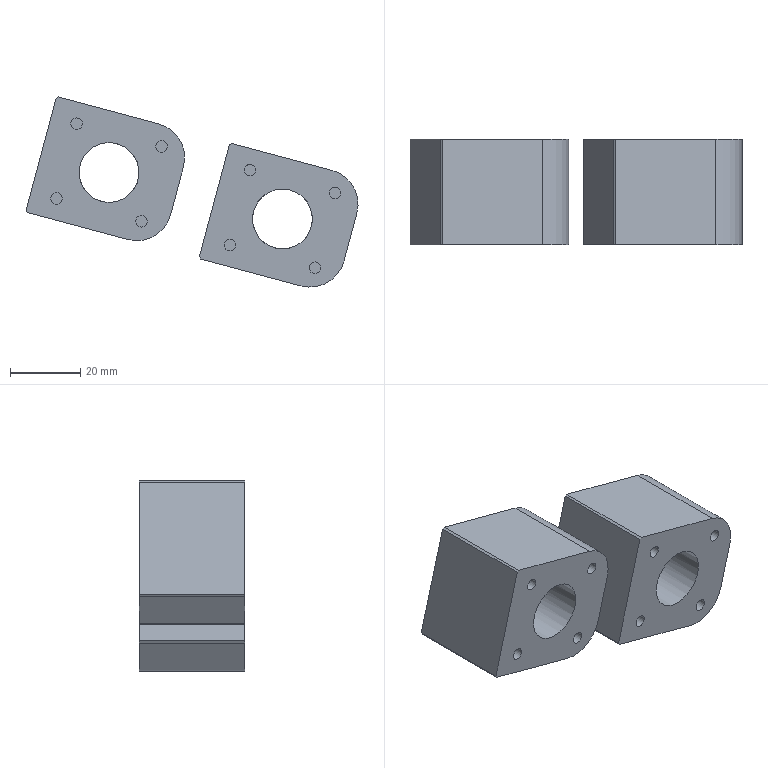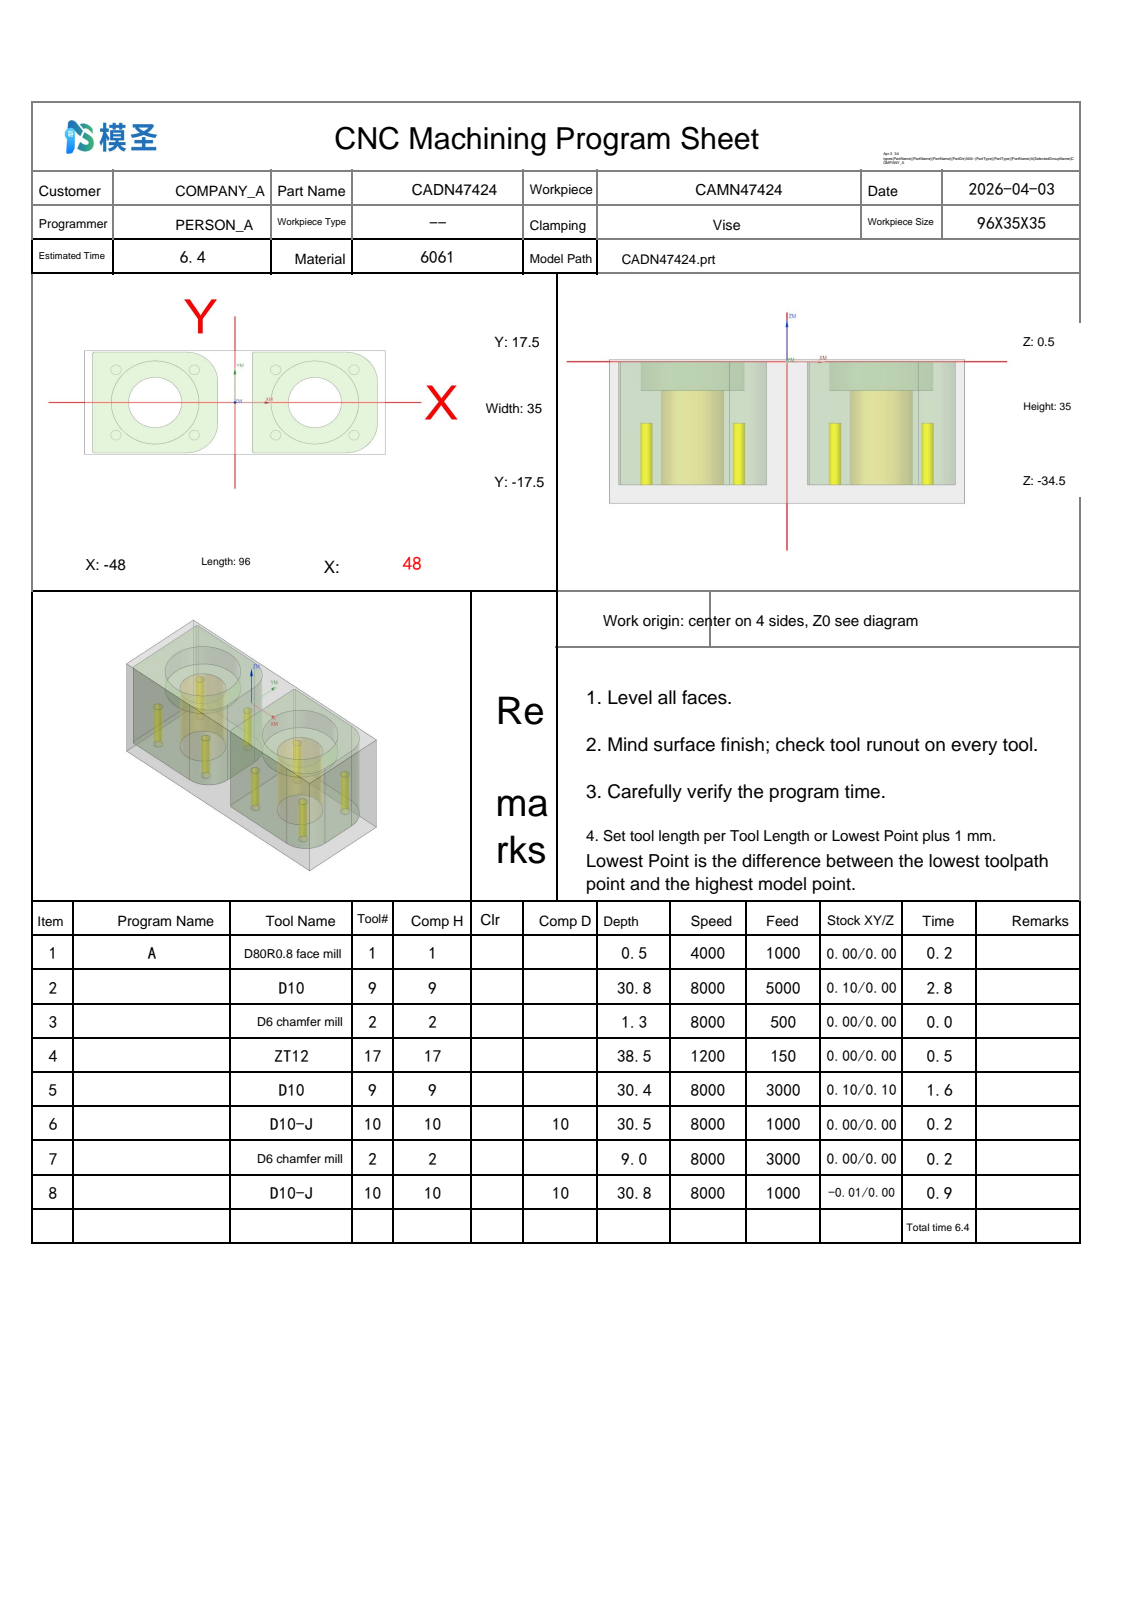NC program | NX | posted by the shop | part box 94.322 x 30 x 54.017 mm
Lines 1 to 1042 of 2047:
%
O0001
(Machine time: 8.07 MIN)
(===Total Tool:5===)
(T1=D80R0.8 face mill D=80.  R=0.8  D-  H01 Z=-0.   )
(T9=D10     D=10.  R=0.   D-  H09 Z=-30.3 )
(T2=D6 chamfer mill   D=6.   R=0.   D-  H02 Z=-8.5  )
(T17=ZT12   D=12.  DR_a=118 D-  H17 Z=-38.  )
(T10=D10-J  D=10.  R=0.   D10 H10 Z=-30.3 )
G80 G90 G17 G49 G40
G91 G28 Z0
M01
N1 T01 M06
(D80R0.8 face mill  D=80. R=0.8 H=01 ce=0.00 di=0.00)
G00 G90 G54 X90.5 Y0.0 M03 S4000
G43 H01 Z20.
M08
Z2.
G01 Z0.0 F1000.
X85.5
X-85.5
X-90.5
Z2.
G00 Z20.
G91 G28 Z0.0
M05
M09
G91 G28 Z0.0
M01
N2 T09 M06
(D10  D=10. R=0. H=09 ce=0.10 di=0.00)
G00 G90 G54 X20.75 Y22.1 M03 S8000
G43 H09 Z20.
M08
Z.5
G01 X35.5 Z.432 F5000.
G02 X50.6 Y7. Z.322 I0.0 J-15.1
G01 Y-7. Z.258
G02 X35.5 Y-22.1 Z.148 I-15.1 J0.0
G01 X6. Z.012
G02 X2.394 Y-20.606 Z-.007 I0.0 J5.1
G01 X1.894 Y-20.106 Z-.01
G02 X.4 Y-16.5 Z-.029 I3.606 J3.606
G01 Y16.5 Z-.181
G02 X1.894 Y20.106 Z-.2 I5.1 J0.0
G01 X2.394 Y20.606 Z-.203
G02 X6. Y22.1 Z-.222 I3.606 J-3.606
G01 X35.5 Z-.358
G02 X50.6 Y7. Z-.468 I0.0 J-15.1
G01 Y-7. Z-.532
G02 X35.5 Y-22.1 Z-.642 I-15.1 J0.0
G01 X6. Z-.778
G02 X2.394 Y-20.606 Z-.797 I0.0 J5.1
G01 X1.894 Y-20.106 Z-.8
G02 X.4 Y-16.5 Z-.819 I3.606 J3.606
G01 Y16.5 Z-.971
G02 X1.894 Y20.106 Z-.99 I5.1 J0.0
G01 X2.394 Y20.606 Z-.993
G02 X6. Y22.1 Z-1.011 I3.606 J-3.606
G01 X35.5 Z-1.148
G02 X50.6 Y7. Z-1.257 I0.0 J-15.1
G01 Y-7. Z-1.322
G02 X35.5 Y-22.1 Z-1.432 I-15.1 J0.0
G01 X6. Z-1.568
G02 X2.394 Y-20.606 Z-1.586 I0.0 J5.1
G01 X1.894 Y-20.106 Z-1.59
G02 X.4 Y-16.5 Z-1.608 I3.606 J3.606
G01 Y16.5 Z-1.761
G02 X1.894 Y20.106 Z-1.779 I5.1 J0.0
G01 X2.394 Y20.606 Z-1.783
G02 X6. Y22.1 Z-1.801 I3.606 J-3.606
G01 X35.5 Z-1.937
G02 X50.6 Y7. Z-2.047 I0.0 J-15.1
G01 Y-7. Z-2.112
G02 X35.5 Y-22.1 Z-2.221 I-15.1 J0.0
G01 X6. Z-2.358
G02 X2.394 Y-20.606 Z-2.376 I0.0 J5.1
G01 X1.894 Y-20.106 Z-2.379
G02 X.4 Y-16.5 Z-2.398 I3.606 J3.606
G01 Y16.5 Z-2.551
G02 X1.894 Y20.106 Z-2.569 I5.1 J0.0
G01 X2.394 Y20.606 Z-2.572
G02 X6. Y22.1 Z-2.591 I3.606 J-3.606
G01 X35.5 Z-2.727
G02 X50.6 Y7. Z-2.837 I0.0 J-15.1
G01 Y-7. Z-2.901
G02 X35.5 Y-22.1 Z-3.011 I-15.1 J0.0
G01 X6. Z-3.147
G02 X2.394 Y-20.606 Z-3.166 I0.0 J5.1
G01 X1.894 Y-20.106 Z-3.169
G02 X.4 Y-16.5 Z-3.188 I3.606 J3.606
G01 Y16.5 Z-3.34
G02 X1.894 Y20.106 Z-3.359 I5.1 J0.0
G01 X2.394 Y20.606 Z-3.362
G02 X6. Y22.1 Z-3.381 I3.606 J-3.606
G01 X35.5 Z-3.517
G02 X50.6 Y7. Z-3.627 I0.0 J-15.1
G01 Y-7. Z-3.691
G02 X35.5 Y-22.1 Z-3.801 I-15.1 J0.0
G01 X6. Z-3.937
G02 X2.394 Y-20.606 Z-3.956 I0.0 J5.1
G01 X1.894 Y-20.106 Z-3.959
G02 X.4 Y-16.5 Z-3.977 I3.606 J3.606
G01 Y16.5 Z-4.13
G02 X1.894 Y20.106 Z-4.149 I5.1 J0.0
G01 X2.394 Y20.606 Z-4.152
G02 X6. Y22.1 Z-4.17 I3.606 J-3.606
G01 X35.5 Z-4.307
G02 X50.6 Y7. Z-4.416 I0.0 J-15.1
G01 Y-7. Z-4.481
G02 X35.5 Y-22.1 Z-4.591 I-15.1 J0.0
G01 X6. Z-4.727
G02 X2.394 Y-20.606 Z-4.745 I0.0 J5.1
G01 X1.894 Y-20.106 Z-4.749
G02 X.4 Y-16.5 Z-4.767 I3.606 J3.606
G01 Y16.5 Z-4.92
G02 X1.894 Y20.106 Z-4.938 I5.1 J0.0
G01 X2.394 Y20.606 Z-4.942
G02 X6. Y22.1 Z-4.96 I3.606 J-3.606
G01 X35.5 Z-5.096
G02 X50.6 Y7. Z-5.206 I0.0 J-15.1
G01 Y-7. Z-5.271
G02 X35.5 Y-22.1 Z-5.38 I-15.1 J0.0
G01 X6. Z-5.517
G02 X2.394 Y-20.606 Z-5.535 I0.0 J5.1
G01 X1.894 Y-20.106 Z-5.538
G02 X.4 Y-16.5 Z-5.557 I3.606 J3.606
G01 Y16.5 Z-5.709
G02 X1.894 Y20.106 Z-5.728 I5.1 J0.0
G01 X2.394 Y20.606 Z-5.731
G02 X6. Y22.1 Z-5.75 I3.606 J-3.606
G01 X35.5 Z-5.886
G02 X50.6 Y7. Z-5.996 I0.0 J-15.1
G01 Y-7. Z-6.06
G02 X35.5 Y-22.1 Z-6.17 I-15.1 J0.0
G01 X6. Z-6.306
G02 X2.394 Y-20.606 Z-6.325 I0.0 J5.1
G01 X1.894 Y-20.106 Z-6.328
G02 X.4 Y-16.5 Z-6.347 I3.606 J3.606
G01 Y16.5 Z-6.499
G02 X1.894 Y20.106 Z-6.518 I5.1 J0.0
G01 X2.394 Y20.606 Z-6.521
G02 X6. Y22.1 Z-6.54 I3.606 J-3.606
G01 X35.5 Z-6.676
G02 X50.6 Y7. Z-6.785 I0.0 J-15.1
G01 Y-7. Z-6.85
G02 X35.5 Y-22.1 Z-6.96 I-15.1 J0.0
G01 X6. Z-7.096
G02 X2.394 Y-20.606 Z-7.115 I0.0 J5.1
G01 X1.894 Y-20.106 Z-7.118
G02 X.4 Y-16.5 Z-7.136 I3.606 J3.606
G01 Y16.5 Z-7.289
G02 X1.894 Y20.106 Z-7.307 I5.1 J0.0
G01 X2.394 Y20.606 Z-7.311
G02 X6. Y22.1 Z-7.329 I3.606 J-3.606
G01 X35.5 Z-7.466
G02 X50.6 Y7. Z-7.575 I0.0 J-15.1
G01 Y-7. Z-7.64
G02 X35.5 Y-22.1 Z-7.75 I-15.1 J0.0
G01 X6. Z-7.886
G02 X2.394 Y-20.606 Z-7.904 I0.0 J5.1
G01 X1.894 Y-20.106 Z-7.908
G02 X.4 Y-16.5 Z-7.926 I3.606 J3.606
G01 Y16.5 Z-8.079
G02 X1.894 Y20.106 Z-8.097 I5.1 J0.0
G01 X2.394 Y20.606 Z-8.1
G02 X6. Y22.1 Z-8.119 I3.606 J-3.606
G01 X35.5 Z-8.255
G02 X50.6 Y7. Z-8.365 I0.0 J-15.1
G01 Y-7. Z-8.43
G02 X35.5 Y-22.1 Z-8.539 I-15.1 J0.0
G01 X6. Z-8.676
G02 X2.394 Y-20.606 Z-8.694 I0.0 J5.1
G01 X1.894 Y-20.106 Z-8.697
G02 X.4 Y-16.5 Z-8.716 I3.606 J3.606
G01 Y16.5 Z-8.868
G02 X1.894 Y20.106 Z-8.887 I5.1 J0.0
G01 X2.394 Y20.606 Z-8.89
G02 X6. Y22.1 Z-8.909 I3.606 J-3.606
G01 X35.5 Z-9.045
G02 X50.6 Y7. Z-9.155 I0.0 J-15.1
G01 Y-7. Z-9.219
G02 X35.5 Y-22.1 Z-9.329 I-15.1 J0.0
G01 X6. Z-9.465
G02 X2.394 Y-20.606 Z-9.484 I0.0 J5.1
G01 X1.894 Y-20.106 Z-9.487
G02 X.4 Y-16.5 Z-9.506 I3.606 J3.606
G01 Y16.5 Z-9.658
G02 X1.894 Y20.106 Z-9.677 I5.1 J0.0
G01 X2.394 Y20.606 Z-9.68
G02 X6. Y22.1 Z-9.698 I3.606 J-3.606
G01 X35.5 Z-9.835
G02 X50.6 Y7. Z-9.944 I0.0 J-15.1
G01 Y-7. Z-10.009
G02 X35.5 Y-22.1 Z-10.119 I-15.1 J0.0
G01 X6. Z-10.255
G02 X2.394 Y-20.606 Z-10.274 I0.0 J5.1
G01 X1.894 Y-20.106 Z-10.277
G02 X.4 Y-16.5 Z-10.295 I3.606 J3.606
G01 Y16.5 Z-10.448
G02 X1.894 Y20.106 Z-10.466 I5.1 J0.0
G01 X2.394 Y20.606 Z-10.47
G02 X6. Y22.1 Z-10.488 I3.606 J-3.606
G01 X35.5 Z-10.625
G02 X50.6 Y7. Z-10.734 I0.0 J-15.1
G01 Y-7. Z-10.799
G02 X35.5 Y-22.1 Z-10.909 I-15.1 J0.0
G01 X6. Z-11.045
G02 X2.394 Y-20.606 Z-11.063 I0.0 J5.1
G01 X1.894 Y-20.106 Z-11.067
G02 X.4 Y-16.5 Z-11.085 I3.606 J3.606
G01 Y16.5 Z-11.238
G02 X1.894 Y20.106 Z-11.256 I5.1 J0.0
G01 X2.394 Y20.606 Z-11.259
G02 X6. Y22.1 Z-11.278 I3.606 J-3.606
G01 X35.5 Z-11.414
G02 X50.6 Y7. Z-11.524 I0.0 J-15.1
G01 Y-7. Z-11.589
G02 X35.5 Y-22.1 Z-11.698 I-15.1 J0.0
G01 X6. Z-11.835
G02 X2.394 Y-20.606 Z-11.853 I0.0 J5.1
G01 X1.894 Y-20.106 Z-11.856
G02 X.4 Y-16.5 Z-11.875 I3.606 J3.606
G01 Y16.5 Z-12.027
G02 X1.894 Y20.106 Z-12.046 I5.1 J0.0
G01 X2.394 Y20.606 Z-12.049
G02 X6. Y22.1 Z-12.068 I3.606 J-3.606
G01 X35.5 Z-12.204
G02 X50.6 Y7. Z-12.314 I0.0 J-15.1
G01 Y-7. Z-12.378
G02 X35.5 Y-22.1 Z-12.488 I-15.1 J0.0
G01 X6. Z-12.624
G02 X2.394 Y-20.606 Z-12.643 I0.0 J5.1
G01 X1.894 Y-20.106 Z-12.646
G02 X.4 Y-16.5 Z-12.665 I3.606 J3.606
G01 Y16.5 Z-12.817
G02 X1.894 Y20.106 Z-12.836 I5.1 J0.0
G01 X2.394 Y20.606 Z-12.839
G02 X6. Y22.1 Z-12.857 I3.606 J-3.606
G01 X35.5 Z-12.994
G02 X50.6 Y7. Z-13.103 I0.0 J-15.1
G01 Y-7. Z-13.168
G02 X35.5 Y-22.1 Z-13.278 I-15.1 J0.0
G01 X6. Z-13.414
G02 X2.394 Y-20.606 Z-13.433 I0.0 J5.1
G01 X1.894 Y-20.106 Z-13.436
G02 X.4 Y-16.5 Z-13.454 I3.606 J3.606
G01 Y16.5 Z-13.607
G02 X1.894 Y20.106 Z-13.625 I5.1 J0.0
G01 X2.394 Y20.606 Z-13.629
G02 X6. Y22.1 Z-13.647 I3.606 J-3.606
G01 X35.5 Z-13.784
G02 X50.6 Y7. Z-13.893 I0.0 J-15.1
G01 Y-7. Z-13.958
G02 X35.5 Y-22.1 Z-14.068 I-15.1 J0.0
G01 X6. Z-14.204
G02 X2.394 Y-20.606 Z-14.222 I0.0 J5.1
G01 X1.894 Y-20.106 Z-14.226
G02 X.4 Y-16.5 Z-14.244 I3.606 J3.606
G01 Y16.5 Z-14.397
G02 X1.894 Y20.106 Z-14.415 I5.1 J0.0
G01 X2.394 Y20.606 Z-14.418
G02 X6. Y22.1 Z-14.437 I3.606 J-3.606
G01 X35.5 Z-14.573
G02 X50.6 Y7. Z-14.683 I0.0 J-15.1
G01 Y-7. Z-14.748
G02 X35.5 Y-22.1 Z-14.857 I-15.1 J0.0
G01 X6. Z-14.994
G02 X2.394 Y-20.606 Z-15.012 I0.0 J5.1
G01 X1.894 Y-20.106 Z-15.015
G02 X.4 Y-16.5 Z-15.034 I3.606 J3.606
G01 Y16.5 Z-15.186
G02 X1.894 Y20.106 Z-15.205 I5.1 J0.0
G01 X2.394 Y20.606 Z-15.208
G02 X6. Y22.1 Z-15.227 I3.606 J-3.606
G01 X35.5 Z-15.363
G02 X50.6 Y7. Z-15.473 I0.0 J-15.1
G01 Y-7. Z-15.537
G02 X35.5 Y-22.1 Z-15.647 I-15.1 J0.0
G01 X6. Z-15.783
G02 X2.394 Y-20.606 Z-15.802 I0.0 J5.1
G01 X1.894 Y-20.106 Z-15.805
G02 X.4 Y-16.5 Z-15.824 I3.606 J3.606
G01 Y16.5 Z-15.976
G02 X1.894 Y20.106 Z-15.995 I5.1 J0.0
G01 X2.394 Y20.606 Z-15.998
G02 X6. Y22.1 Z-16.016 I3.606 J-3.606
G01 X35.5 Z-16.153
G02 X50.6 Y7. Z-16.262 I0.0 J-15.1
G01 Y-7. Z-16.327
G02 X35.5 Y-22.1 Z-16.437 I-15.1 J0.0
G01 X6. Z-16.573
G02 X2.394 Y-20.606 Z-16.592 I0.0 J5.1
G01 X1.894 Y-20.106 Z-16.595
G02 X.4 Y-16.5 Z-16.613 I3.606 J3.606
G01 Y16.5 Z-16.766
G02 X1.894 Y20.106 Z-16.784 I5.1 J0.0
G01 X2.394 Y20.606 Z-16.788
G02 X6. Y22.1 Z-16.806 I3.606 J-3.606
G01 X35.5 Z-16.943
G02 X50.6 Y7. Z-17.052 I0.0 J-15.1
G01 Y-7. Z-17.117
G02 X35.5 Y-22.1 Z-17.226 I-15.1 J0.0
G01 X6. Z-17.363
G02 X2.394 Y-20.606 Z-17.381 I0.0 J5.1
G01 X1.894 Y-20.106 Z-17.385
G02 X.4 Y-16.5 Z-17.403 I3.606 J3.606
G01 Y16.5 Z-17.556
G02 X1.894 Y20.106 Z-17.574 I5.1 J0.0
G01 X2.394 Y20.606 Z-17.577
G02 X6. Y22.1 Z-17.596 I3.606 J-3.606
G01 X35.5 Z-17.732
G02 X50.6 Y7. Z-17.842 I0.0 J-15.1
G01 Y-7. Z-17.907
G02 X35.5 Y-22.1 Z-18.016 I-15.1 J0.0
G01 X6. Z-18.153
G02 X2.394 Y-20.606 Z-18.171 I0.0 J5.1
G01 X1.894 Y-20.106 Z-18.174
G02 X.4 Y-16.5 Z-18.193 I3.606 J3.606
G01 Y16.5 Z-18.345
G02 X1.894 Y20.106 Z-18.364 I5.1 J0.0
G01 X2.394 Y20.606 Z-18.367
G02 X6. Y22.1 Z-18.386 I3.606 J-3.606
G01 X35.5 Z-18.522
G02 X50.6 Y7. Z-18.632 I0.0 J-15.1
G01 Y-7. Z-18.696
G02 X35.5 Y-22.1 Z-18.806 I-15.1 J0.0
G01 X6. Z-18.942
G02 X2.394 Y-20.606 Z-18.961 I0.0 J5.1
G01 X1.894 Y-20.106 Z-18.964
G02 X.4 Y-16.5 Z-18.983 I3.606 J3.606
G01 Y16.5 Z-19.135
G02 X1.894 Y20.106 Z-19.154 I5.1 J0.0
G01 X2.394 Y20.606 Z-19.157
G02 X6. Y22.1 Z-19.175 I3.606 J-3.606
G01 X35.5 Z-19.312
G02 X50.6 Y7. Z-19.421 I0.0 J-15.1
G01 Y-7. Z-19.486
G02 X35.5 Y-22.1 Z-19.596 I-15.1 J0.0
G01 X6. Z-19.732
G02 X2.394 Y-20.606 Z-19.751 I0.0 J5.1
G01 X1.894 Y-20.106 Z-19.754
G02 X.4 Y-16.5 Z-19.772 I3.606 J3.606
G01 Y16.5 Z-19.925
G02 X1.894 Y20.106 Z-19.943 I5.1 J0.0
G01 X2.394 Y20.606 Z-19.947
G02 X6. Y22.1 Z-19.965 I3.606 J-3.606
G01 X35.5 Z-20.102
G02 X50.6 Y7. Z-20.211 I0.0 J-15.1
G01 Y-7. Z-20.276
G02 X35.5 Y-22.1 Z-20.385 I-15.1 J0.0
G01 X6. Z-20.522
G02 X2.394 Y-20.606 Z-20.54 I0.0 J5.1
G01 X1.894 Y-20.106 Z-20.544
G02 X.4 Y-16.5 Z-20.562 I3.606 J3.606
G01 Y16.5 Z-20.715
G02 X1.894 Y20.106 Z-20.733 I5.1 J0.0
G01 X2.394 Y20.606 Z-20.736
G02 X6. Y22.1 Z-20.755 I3.606 J-3.606
G01 X35.5 Z-20.891
G02 X50.6 Y7. Z-21.001 I0.0 J-15.1
G01 Y-7. Z-21.066
G02 X35.5 Y-22.1 Z-21.175 I-15.1 J0.0
G01 X6. Z-21.312
G02 X2.394 Y-20.606 Z-21.33 I0.0 J5.1
G01 X1.894 Y-20.106 Z-21.333
G02 X.4 Y-16.5 Z-21.352 I3.606 J3.606
G01 Y16.5 Z-21.504
G02 X1.894 Y20.106 Z-21.523 I5.1 J0.0
G01 X2.394 Y20.606 Z-21.526
G02 X6. Y22.1 Z-21.545 I3.606 J-3.606
G01 X35.5 Z-21.681
G02 X50.6 Y7. Z-21.791 I0.0 J-15.1
G01 Y-7. Z-21.855
G02 X35.5 Y-22.1 Z-21.965 I-15.1 J0.0
G01 X6. Z-22.101
G02 X2.394 Y-20.606 Z-22.12 I0.0 J5.1
G01 X1.894 Y-20.106 Z-22.123
G02 X.4 Y-16.5 Z-22.142 I3.606 J3.606
G01 Y16.5 Z-22.294
G02 X1.894 Y20.106 Z-22.313 I5.1 J0.0
G01 X2.394 Y20.606 Z-22.316
G02 X6. Y22.1 Z-22.334 I3.606 J-3.606
G01 X35.5 Z-22.471
G02 X50.6 Y7. Z-22.58 I0.0 J-15.1
G01 Y-7. Z-22.645
G02 X35.5 Y-22.1 Z-22.755 I-15.1 J0.0
G01 X6. Z-22.891
G02 X2.394 Y-20.606 Z-22.91 I0.0 J5.1
G01 X1.894 Y-20.106 Z-22.913
G02 X.4 Y-16.5 Z-22.931 I3.606 J3.606
G01 Y16.5 Z-23.084
G02 X1.894 Y20.106 Z-23.102 I5.1 J0.0
G01 X2.394 Y20.606 Z-23.106
G02 X6. Y22.1 Z-23.124 I3.606 J-3.606
G01 X35.5 Z-23.26
G02 X50.6 Y7. Z-23.37 I0.0 J-15.1
G01 Y-7. Z-23.435
G02 X35.5 Y-22.1 Z-23.544 I-15.1 J0.0
G01 X6. Z-23.681
G02 X2.394 Y-20.606 Z-23.699 I0.0 J5.1
G01 X1.894 Y-20.106 Z-23.703
G02 X.4 Y-16.5 Z-23.721 I3.606 J3.606
G01 Y16.5 Z-23.874
G02 X1.894 Y20.106 Z-23.892 I5.1 J0.0
G01 X2.394 Y20.606 Z-23.895
G02 X6. Y22.1 Z-23.914 I3.606 J-3.606
G01 X35.5 Z-24.05
G02 X50.6 Y7. Z-24.16 I0.0 J-15.1
G01 Y-7. Z-24.225
G02 X35.5 Y-22.1 Z-24.334 I-15.1 J0.0
G01 X6. Z-24.471
G02 X2.394 Y-20.606 Z-24.489 I0.0 J5.1
G01 X1.894 Y-20.106 Z-24.492
G02 X.4 Y-16.5 Z-24.511 I3.606 J3.606
G01 Y16.5 Z-24.663
G02 X1.894 Y20.106 Z-24.682 I5.1 J0.0
G01 X2.394 Y20.606 Z-24.685
G02 X6. Y22.1 Z-24.704 I3.606 J-3.606
G01 X35.5 Z-24.84
G02 X50.6 Y7. Z-24.95 I0.0 J-15.1
G01 Y-7. Z-25.014
G02 X35.5 Y-22.1 Z-25.124 I-15.1 J0.0
G01 X6. Z-25.26
G02 X2.394 Y-20.606 Z-25.279 I0.0 J5.1
G01 X1.894 Y-20.106 Z-25.282
G02 X.4 Y-16.5 Z-25.301 I3.606 J3.606
G01 Y16.5 Z-25.453
G02 X1.894 Y20.106 Z-25.472 I5.1 J0.0
G01 X2.394 Y20.606 Z-25.475
G02 X6. Y22.1 Z-25.493 I3.606 J-3.606
G01 X35.5 Z-25.63
G02 X50.6 Y7. Z-25.739 I0.0 J-15.1
G01 Y-7. Z-25.804
G02 X35.5 Y-22.1 Z-25.914 I-15.1 J0.0
G01 X6. Z-26.05
G02 X2.394 Y-20.606 Z-26.069 I0.0 J5.1
G01 X1.894 Y-20.106 Z-26.072
G02 X.4 Y-16.5 Z-26.09 I3.606 J3.606
G01 Y16.5 Z-26.243
G02 X1.894 Y20.106 Z-26.261 I5.1 J0.0
G01 X2.394 Y20.606 Z-26.265
G02 X6. Y22.1 Z-26.283 I3.606 J-3.606
G01 X35.5 Z-26.419
G02 X50.6 Y7. Z-26.529 I0.0 J-15.1
G01 Y-7. Z-26.594
G02 X35.5 Y-22.1 Z-26.703 I-15.1 J0.0
G01 X6. Z-26.84
G02 X2.394 Y-20.606 Z-26.858 I0.0 J5.1
G01 X1.894 Y-20.106 Z-26.862
G02 X.4 Y-16.5 Z-26.88 I3.606 J3.606
G01 Y16.5 Z-27.033
G02 X1.894 Y20.106 Z-27.051 I5.1 J0.0
G01 X2.394 Y20.606 Z-27.054
G02 X6. Y22.1 Z-27.073 I3.606 J-3.606
G01 X35.5 Z-27.209
G02 X50.6 Y7. Z-27.319 I0.0 J-15.1
G01 Y-7. Z-27.384
G02 X35.5 Y-22.1 Z-27.493 I-15.1 J0.0
G01 X6. Z-27.629
G02 X2.394 Y-20.606 Z-27.648 I0.0 J5.1
G01 X1.894 Y-20.106 Z-27.651
G02 X.4 Y-16.5 Z-27.67 I3.606 J3.606
G01 Y16.5 Z-27.822
G02 X1.894 Y20.106 Z-27.841 I5.1 J0.0
G01 X2.394 Y20.606 Z-27.844
G02 X6. Y22.1 Z-27.863 I3.606 J-3.606
G01 X35.5 Z-27.999
G02 X50.6 Y7. Z-28.109 I0.0 J-15.1
G01 Y-7. Z-28.173
G02 X35.5 Y-22.1 Z-28.283 I-15.1 J0.0
G01 X6. Z-28.419
G02 X2.394 Y-20.606 Z-28.438 I0.0 J5.1
G01 X1.894 Y-20.106 Z-28.441
G02 X.4 Y-16.5 Z-28.46 I3.606 J3.606
G01 Y16.5 Z-28.612
G02 X1.894 Y20.106 Z-28.631 I5.1 J0.0
G01 X2.394 Y20.606 Z-28.634
G02 X6. Y22.1 Z-28.652 I3.606 J-3.606
G01 X35.5 Z-28.789
G02 X50.6 Y7. Z-28.898 I0.0 J-15.1
G01 Y-7. Z-28.963
G02 X35.5 Y-22.1 Z-29.073 I-15.1 J0.0
G01 X6. Z-29.209
G02 X2.394 Y-20.606 Z-29.227 I0.0 J5.1
G01 X1.894 Y-20.106 Z-29.231
G02 X.4 Y-16.5 Z-29.249 I3.606 J3.606
G01 Y16.5 Z-29.402
G02 X1.894 Y20.106 Z-29.42 I5.1 J0.0
G01 X2.394 Y20.606 Z-29.424
G02 X6. Y22.1 Z-29.442 I3.606 J-3.606
G01 X35.5 Z-29.578
G02 X50.6 Y7. Z-29.688 I0.0 J-15.1
G01 Y-7. Z-29.753
G02 X35.5 Y-22.1 Z-29.862 I-15.1 J0.0
G01 X6. Z-29.999
G02 X2.394 Y-20.606 Z-30.017 I0.0 J5.1
G01 X1.894 Y-20.106 Z-30.021
G02 X.4 Y-16.5 Z-30.039 I3.606 J3.606
G01 Y16.5 Z-30.192
G02 X1.894 Y20.106 Z-30.21 I5.1 J0.0
G01 X2.394 Y20.606 Z-30.213
G02 X6. Y22.1 Z-30.232 I3.606 J-3.606
G01 X20.75 Z-30.3
X35.5
G02 X50.6 Y7. I0.0 J-15.1
G01 Y-7.
G02 X35.5 Y-22.1 I-15.1 J0.0
G01 X6.
G02 X2.394 Y-20.606 I0.0 J5.1
G01 X1.894 Y-20.106
G02 X.4 Y-16.5 I3.606 J3.606
G01 Y16.5
G02 X1.894 Y20.106 I5.1 J0.0
G01 X2.394 Y20.606
G02 X6. Y22.1 I3.606 J-3.606
G01 X20.75
X21.25
Z-29.3
G00 Z20.
X-50.6 Y0.0
Z.5
G01 Y16.5 Z.424
G02 X-49.106 Y20.106 Z.405 I5.1 J0.0
G01 X-48.606 Y20.606 Z.402
G02 X-45. Y22.1 Z.383 I3.606 J-3.606
G01 X-15.5 Z.247
G02 X-.4 Y7. Z.137 I0.0 J-15.1
G01 Y-7. Z.073
G02 X-15.5 Y-22.1 Z-.037 I-15.1 J0.0
G01 X-45. Z-.173
G02 X-48.606 Y-20.606 Z-.192 I0.0 J5.1
G01 X-49.106 Y-20.106 Z-.195
G02 X-50.6 Y-16.5 Z-.213 I3.606 J3.606
G01 Y16.5 Z-.366
G02 X-49.106 Y20.106 Z-.385 I5.1 J0.0
G01 X-48.606 Y20.606 Z-.388
G02 X-45. Y22.1 Z-.406 I3.606 J-3.606
G01 X-15.5 Z-.543
G02 X-.4 Y7. Z-.652 I0.0 J-15.1
G01 Y-7. Z-.717
G02 X-15.5 Y-22.1 Z-.827 I-15.1 J0.0
G01 X-45. Z-.963
G02 X-48.606 Y-20.606 Z-.981 I0.0 J5.1
G01 X-49.106 Y-20.106 Z-.985
G02 X-50.6 Y-16.5 Z-1.003 I3.606 J3.606
G01 Y16.5 Z-1.156
G02 X-49.106 Y20.106 Z-1.174 I5.1 J0.0
G01 X-48.606 Y20.606 Z-1.178
G02 X-45. Y22.1 Z-1.196 I3.606 J-3.606
G01 X-15.5 Z-1.332
G02 X-.4 Y7. Z-1.442 I0.0 J-15.1
G01 Y-7. Z-1.507
G02 X-15.5 Y-22.1 Z-1.616 I-15.1 J0.0
G01 X-45. Z-1.753
G02 X-48.606 Y-20.606 Z-1.771 I0.0 J5.1
G01 X-49.106 Y-20.106 Z-1.774
G02 X-50.6 Y-16.5 Z-1.793 I3.606 J3.606
G01 Y16.5 Z-1.945
G02 X-49.106 Y20.106 Z-1.964 I5.1 J0.0
G01 X-48.606 Y20.606 Z-1.967
G02 X-45. Y22.1 Z-1.986 I3.606 J-3.606
G01 X-15.5 Z-2.122
G02 X-.4 Y7. Z-2.232 I0.0 J-15.1
G01 Y-7. Z-2.296
G02 X-15.5 Y-22.1 Z-2.406 I-15.1 J0.0
G01 X-45. Z-2.542
G02 X-48.606 Y-20.606 Z-2.561 I0.0 J5.1
G01 X-49.106 Y-20.106 Z-2.564
G02 X-50.6 Y-16.5 Z-2.583 I3.606 J3.606
G01 Y16.5 Z-2.735
G02 X-49.106 Y20.106 Z-2.754 I5.1 J0.0
G01 X-48.606 Y20.606 Z-2.757
G02 X-45. Y22.1 Z-2.776 I3.606 J-3.606
G01 X-15.5 Z-2.912
G02 X-.4 Y7. Z-3.021 I0.0 J-15.1
G01 Y-7. Z-3.086
G02 X-15.5 Y-22.1 Z-3.196 I-15.1 J0.0
G01 X-45. Z-3.332
G02 X-48.606 Y-20.606 Z-3.351 I0.0 J5.1
G01 X-49.106 Y-20.106 Z-3.354
G02 X-50.6 Y-16.5 Z-3.372 I3.606 J3.606
G01 Y16.5 Z-3.525
G02 X-49.106 Y20.106 Z-3.543 I5.1 J0.0
G01 X-48.606 Y20.606 Z-3.547
G02 X-45. Y22.1 Z-3.565 I3.606 J-3.606
G01 X-15.5 Z-3.702
G02 X-.4 Y7. Z-3.811 I0.0 J-15.1
G01 Y-7. Z-3.876
G02 X-15.5 Y-22.1 Z-3.986 I-15.1 J0.0
G01 X-45. Z-4.122
G02 X-48.606 Y-20.606 Z-4.14 I0.0 J5.1
G01 X-49.106 Y-20.106 Z-4.144
G02 X-50.6 Y-16.5 Z-4.162 I3.606 J3.606
G01 Y16.5 Z-4.315
G02 X-49.106 Y20.106 Z-4.333 I5.1 J0.0
G01 X-48.606 Y20.606 Z-4.337
G02 X-45. Y22.1 Z-4.355 I3.606 J-3.606
G01 X-15.5 Z-4.491
G02 X-.4 Y7. Z-4.601 I0.0 J-15.1
G01 Y-7. Z-4.666
G02 X-15.5 Y-22.1 Z-4.775 I-15.1 J0.0
G01 X-45. Z-4.912
G02 X-48.606 Y-20.606 Z-4.93 I0.0 J5.1
G01 X-49.106 Y-20.106 Z-4.933
G02 X-50.6 Y-16.5 Z-4.952 I3.606 J3.606
G01 Y16.5 Z-5.104
G02 X-49.106 Y20.106 Z-5.123 I5.1 J0.0
G01 X-48.606 Y20.606 Z-5.126
G02 X-45. Y22.1 Z-5.145 I3.606 J-3.606
G01 X-15.5 Z-5.281
G02 X-.4 Y7. Z-5.391 I0.0 J-15.1
G01 Y-7. Z-5.455
G02 X-15.5 Y-22.1 Z-5.565 I-15.1 J0.0
G01 X-45. Z-5.701
G02 X-48.606 Y-20.606 Z-5.72 I0.0 J5.1
G01 X-49.106 Y-20.106 Z-5.723
G02 X-50.6 Y-16.5 Z-5.742 I3.606 J3.606
G01 Y16.5 Z-5.894
G02 X-49.106 Y20.106 Z-5.913 I5.1 J0.0
G01 X-48.606 Y20.606 Z-5.916
G02 X-45. Y22.1 Z-5.935 I3.606 J-3.606
G01 X-15.5 Z-6.071
G02 X-.4 Y7. Z-6.18 I0.0 J-15.1
G01 Y-7. Z-6.245
G02 X-15.5 Y-22.1 Z-6.355 I-15.1 J0.0
G01 X-45. Z-6.491
G02 X-48.606 Y-20.606 Z-6.51 I0.0 J5.1
G01 X-49.106 Y-20.106 Z-6.513
G02 X-50.6 Y-16.5 Z-6.531 I3.606 J3.606
G01 Y16.5 Z-6.684
G02 X-49.106 Y20.106 Z-6.702 I5.1 J0.0
G01 X-48.606 Y20.606 Z-6.706
G02 X-45. Y22.1 Z-6.724 I3.606 J-3.606
G01 X-15.5 Z-6.861
G02 X-.4 Y7. Z-6.97 I0.0 J-15.1
G01 Y-7. Z-7.035
G02 X-15.5 Y-22.1 Z-7.145 I-15.1 J0.0
G01 X-45. Z-7.281
G02 X-48.606 Y-20.606 Z-7.299 I0.0 J5.1
G01 X-49.106 Y-20.106 Z-7.303
G02 X-50.6 Y-16.5 Z-7.321 I3.606 J3.606
G01 Y16.5 Z-7.474
G02 X-49.106 Y20.106 Z-7.492 I5.1 J0.0
G01 X-48.606 Y20.606 Z-7.495
G02 X-45. Y22.1 Z-7.514 I3.606 J-3.606
G01 X-15.5 Z-7.65
G02 X-.4 Y7. Z-7.76 I0.0 J-15.1
G01 Y-7. Z-7.825
G02 X-15.5 Y-22.1 Z-7.934 I-15.1 J0.0
G01 X-45. Z-8.071
G02 X-48.606 Y-20.606 Z-8.089 I0.0 J5.1
G01 X-49.106 Y-20.106 Z-8.092
G02 X-50.6 Y-16.5 Z-8.111 I3.606 J3.606
G01 Y16.5 Z-8.263
G02 X-49.106 Y20.106 Z-8.282 I5.1 J0.0
G01 X-48.606 Y20.606 Z-8.285
G02 X-45. Y22.1 Z-8.304 I3.606 J-3.606
G01 X-15.5 Z-8.44
G02 X-.4 Y7. Z-8.55 I0.0 J-15.1
G01 Y-7. Z-8.614
G02 X-15.5 Y-22.1 Z-8.724 I-15.1 J0.0
G01 X-45. Z-8.86
G02 X-48.606 Y-20.606 Z-8.879 I0.0 J5.1
G01 X-49.106 Y-20.106 Z-8.882
G02 X-50.6 Y-16.5 Z-8.901 I3.606 J3.606
G01 Y16.5 Z-9.053
G02 X-49.106 Y20.106 Z-9.072 I5.1 J0.0
G01 X-48.606 Y20.606 Z-9.075
G02 X-45. Y22.1 Z-9.093 I3.606 J-3.606
G01 X-15.5 Z-9.23
G02 X-.4 Y7. Z-9.339 I0.0 J-15.1
G01 Y-7. Z-9.404
G02 X-15.5 Y-22.1 Z-9.514 I-15.1 J0.0
G01 X-45. Z-9.65
G02 X-48.606 Y-20.606 Z-9.669 I0.0 J5.1
G01 X-49.106 Y-20.106 Z-9.672
G02 X-50.6 Y-16.5 Z-9.69 I3.606 J3.606
G01 Y16.5 Z-9.843
G02 X-49.106 Y20.106 Z-9.861 I5.1 J0.0
G01 X-48.606 Y20.606 Z-9.865
G02 X-45. Y22.1 Z-9.883 I3.606 J-3.606
G01 X-15.5 Z-10.02
G02 X-.4 Y7. Z-10.129 I0.0 J-15.1
G01 Y-7. Z-10.194
G02 X-15.5 Y-22.1 Z-10.304 I-15.1 J0.0
G01 X-45. Z-10.44
G02 X-48.606 Y-20.606 Z-10.458 I0.0 J5.1
G01 X-49.106 Y-20.106 Z-10.462
G02 X-50.6 Y-16.5 Z-10.48 I3.606 J3.606
G01 Y16.5 Z-10.633
G02 X-49.106 Y20.106 Z-10.651 I5.1 J0.0
G01 X-48.606 Y20.606 Z-10.654
G02 X-45. Y22.1 Z-10.673 I3.606 J-3.606
G01 X-15.5 Z-10.809
G02 X-.4 Y7. Z-10.919 I0.0 J-15.1
G01 Y-7. Z-10.984
G02 X-15.5 Y-22.1 Z-11.093 I-15.1 J0.0
G01 X-45. Z-11.23
G02 X-48.606 Y-20.606 Z-11.248 I0.0 J5.1
G01 X-49.106 Y-20.106 Z-11.251
G02 X-50.6 Y-16.5 Z-11.27 I3.606 J3.606
G01 Y16.5 Z-11.422
G02 X-49.106 Y20.106 Z-11.441 I5.1 J0.0
G01 X-48.606 Y20.606 Z-11.444
G02 X-45. Y22.1 Z-11.463 I3.606 J-3.606
G01 X-15.5 Z-11.599
G02 X-.4 Y7. Z-11.709 I0.0 J-15.1
G01 Y-7. Z-11.773
G02 X-15.5 Y-22.1 Z-11.883 I-15.1 J0.0
G01 X-45. Z-12.019
G02 X-48.606 Y-20.606 Z-12.038 I0.0 J5.1
G01 X-49.106 Y-20.106 Z-12.041
G02 X-50.6 Y-16.5 Z-12.06 I3.606 J3.606
G01 Y16.5 Z-12.212
G02 X-49.106 Y20.106 Z-12.231 I5.1 J0.0
G01 X-48.606 Y20.606 Z-12.234
G02 X-45. Y22.1 Z-12.252 I3.606 J-3.606
G01 X-15.5 Z-12.389
G02 X-.4 Y7. Z-12.498 I0.0 J-15.1
G01 Y-7. Z-12.563
G02 X-15.5 Y-22.1 Z-12.673 I-15.1 J0.0
G01 X-45. Z-12.809
G02 X-48.606 Y-20.606 Z-12.828 I0.0 J5.1
G01 X-49.106 Y-20.106 Z-12.831
G02 X-50.6 Y-16.5 Z-12.849 I3.606 J3.606
G01 Y16.5 Z-13.002
G02 X-49.106 Y20.106 Z-13.02 I5.1 J0.0
G01 X-48.606 Y20.606 Z-13.024
G02 X-45. Y22.1 Z-13.042 I3.606 J-3.606
G01 X-15.5 Z-13.179
G02 X-.4 Y7. Z-13.288 I0.0 J-15.1
G01 Y-7. Z-13.353
G02 X-15.5 Y-22.1 Z-13.462 I-15.1 J0.0
G01 X-45. Z-13.599
G02 X-48.606 Y-20.606 Z-13.617 I0.0 J5.1
G01 X-49.106 Y-20.106 Z-13.621
G02 X-50.6 Y-16.5 Z-13.639 I3.606 J3.606
G01 Y16.5 Z-13.792
G02 X-49.106 Y20.106 Z-13.81 I5.1 J0.0
G01 X-48.606 Y20.606 Z-13.813
G02 X-45. Y22.1 Z-13.832 I3.606 J-3.606
G01 X-15.5 Z-13.968
G02 X-.4 Y7. Z-14.078 I0.0 J-15.1
G01 Y-7. Z-14.143
G02 X-15.5 Y-22.1 Z-14.252 I-15.1 J0.0
G01 X-45. Z-14.389
G02 X-48.606 Y-20.606 Z-14.407 I0.0 J5.1
G01 X-49.106 Y-20.106 Z-14.41
G02 X-50.6 Y-16.5 Z-14.429 I3.606 J3.606
G01 Y16.5 Z-14.581
G02 X-49.106 Y20.106 Z-14.6 I5.1 J0.0
G01 X-48.606 Y20.606 Z-14.603
G02 X-45. Y22.1 Z-14.622 I3.606 J-3.606
G01 X-15.5 Z-14.758
G02 X-.4 Y7. Z-14.868 I0.0 J-15.1
G01 Y-7. Z-14.932
G02 X-15.5 Y-22.1 Z-15.042 I-15.1 J0.0
G01 X-45. Z-15.178
G02 X-48.606 Y-20.606 Z-15.197 I0.0 J5.1
G01 X-49.106 Y-20.106 Z-15.2
G02 X-50.6 Y-16.5 Z-15.219 I3.606 J3.606
G01 Y16.5 Z-15.371
G02 X-49.106 Y20.106 Z-15.39 I5.1 J0.0
G01 X-48.606 Y20.606 Z-15.393
G02 X-45. Y22.1 Z-15.411 I3.606 J-3.606
G01 X-15.5 Z-15.548
G02 X-.4 Y7. Z-15.657 I0.0 J-15.1
G01 Y-7. Z-15.722
G02 X-15.5 Y-22.1 Z-15.832 I-15.1 J0.0
G01 X-45. Z-15.968
G02 X-48.606 Y-20.606 Z-15.987 I0.0 J5.1
G01 X-49.106 Y-20.106 Z-15.99
G02 X-50.6 Y-16.5 Z-16.008 I3.606 J3.606
G01 Y16.5 Z-16.161
G02 X-49.106 Y20.106 Z-16.179 I5.1 J0.0
G01 X-48.606 Y20.606 Z-16.183
G02 X-45. Y22.1 Z-16.201 I3.606 J-3.606
G01 X-15.5 Z-16.338
G02 X-.4 Y7. Z-16.447 I0.0 J-15.1
G01 Y-7. Z-16.512
G02 X-15.5 Y-22.1 Z-16.621 I-15.1 J0.0
G01 X-45. Z-16.758
G02 X-48.606 Y-20.606 Z-16.776 I0.0 J5.1
G01 X-49.106 Y-20.106 Z-16.78
G02 X-50.6 Y-16.5 Z-16.798 I3.606 J3.606
G01 Y16.5 Z-16.951
G02 X-49.106 Y20.106 Z-16.969 I5.1 J0.0
G01 X-48.606 Y20.606 Z-16.972
G02 X-45. Y22.1 Z-16.991 I3.606 J-3.606
G01 X-15.5 Z-17.127
G02 X-.4 Y7. Z-17.237 I0.0 J-15.1
G01 Y-7. Z-17.302
G02 X-15.5 Y-22.1 Z-17.411 I-15.1 J0.0
G01 X-45. Z-17.548
G02 X-48.606 Y-20.606 Z-17.566 I0.0 J5.1
G01 X-49.106 Y-20.106 Z-17.569
G02 X-50.6 Y-16.5 Z-17.588 I3.606 J3.606
G01 Y16.5 Z-17.74
G02 X-49.106 Y20.106 Z-17.759 I5.1 J0.0
G01 X-48.606 Y20.606 Z-17.762
G02 X-45. Y22.1 Z-17.781 I3.606 J-3.606
G01 X-15.5 Z-17.917
G02 X-.4 Y7. Z-18.027 I0.0 J-15.1
G01 Y-7. Z-18.091
G02 X-15.5 Y-22.1 Z-18.201 I-15.1 J0.0
G01 X-45. Z-18.337
G02 X-48.606 Y-20.606 Z-18.356 I0.0 J5.1
G01 X-49.106 Y-20.106 Z-18.359
G02 X-50.6 Y-16.5 Z-18.378 I3.606 J3.606
G01 Y16.5 Z-18.53
G02 X-49.106 Y20.106 Z-18.549 I5.1 J0.0
G01 X-48.606 Y20.606 Z-18.552
G02 X-45. Y22.1 Z-18.57 I3.606 J-3.606
G01 X-15.5 Z-18.707
G02 X-.4 Y7. Z-18.816 I0.0 J-15.1
G01 Y-7. Z-18.881
G02 X-15.5 Y-22.1 Z-18.991 I-15.1 J0.0
G01 X-45. Z-19.127
G02 X-48.606 Y-20.606 Z-19.146 I0.0 J5.1
G01 X-49.106 Y-20.106 Z-19.149
G02 X-50.6 Y-16.5 Z-19.167 I3.606 J3.606
G01 Y16.5 Z-19.32
G02 X-49.106 Y20.106 Z-19.338 I5.1 J0.0
G01 X-48.606 Y20.606 Z-19.342
G02 X-45. Y22.1 Z-19.36 I3.606 J-3.606
G01 X-15.5 Z-19.496
G02 X-.4 Y7. Z-19.606 I0.0 J-15.1
G01 Y-7. Z-19.671
G02 X-15.5 Y-22.1 Z-19.78 I-15.1 J0.0
G01 X-45. Z-19.917
G02 X-48.606 Y-20.606 Z-19.935 I0.0 J5.1
G01 X-49.106 Y-20.106 Z-19.939
G02 X-50.6 Y-16.5 Z-19.957 I3.606 J3.606
G01 Y16.5 Z-20.11
G02 X-49.106 Y20.106 Z-20.128 I5.1 J0.0
G01 X-48.606 Y20.606 Z-20.131
G02 X-45. Y22.1 Z-20.15 I3.606 J-3.606
G01 X-15.5 Z-20.286
G02 X-.4 Y7. Z-20.396 I0.0 J-15.1
G01 Y-7. Z-20.461
G02 X-15.5 Y-22.1 Z-20.57 I-15.1 J0.0
G01 X-45. Z-20.707
G02 X-48.606 Y-20.606 Z-20.725 I0.0 J5.1
G01 X-49.106 Y-20.106 Z-20.728
G02 X-50.6 Y-16.5 Z-20.747 I3.606 J3.606
G01 Y16.5 Z-20.899
G02 X-49.106 Y20.106 Z-20.918 I5.1 J0.0
G01 X-48.606 Y20.606 Z-20.921
G02 X-45. Y22.1 Z-20.94 I3.606 J-3.606
G01 X-15.5 Z-21.076
G02 X-.4 Y7. Z-21.186 I0.0 J-15.1
G01 Y-7. Z-21.25
G02 X-15.5 Y-22.1 Z-21.36 I-15.1 J0.0
G01 X-45. Z-21.496
G02 X-48.606 Y-20.606 Z-21.515 I0.0 J5.1
G01 X-49.106 Y-20.106 Z-21.518
G02 X-50.6 Y-16.5 Z-21.537 I3.606 J3.606
G01 Y16.5 Z-21.689
G02 X-49.106 Y20.106 Z-21.708 I5.1 J0.0
G01 X-48.606 Y20.606 Z-21.711
G02 X-45. Y22.1 Z-21.729 I3.606 J-3.606
G01 X-15.5 Z-21.866
G02 X-.4 Y7. Z-21.975 I0.0 J-15.1
G01 Y-7. Z-22.04
G02 X-15.5 Y-22.1 Z-22.15 I-15.1 J0.0
G01 X-45. Z-22.286
G02 X-48.606 Y-20.606 Z-22.305 I0.0 J5.1
G01 X-49.106 Y-20.106 Z-22.308
G02 X-50.6 Y-16.5 Z-22.326 I3.606 J3.606
G01 Y16.5 Z-22.479
G02 X-49.106 Y20.106 Z-22.497 I5.1 J0.0
G01 X-48.606 Y20.606 Z-22.501
G02 X-45. Y22.1 Z-22.519 I3.606 J-3.606
G01 X-15.5 Z-22.655
G02 X-.4 Y7. Z-22.765 I0.0 J-15.1
G01 Y-7. Z-22.83
G02 X-15.5 Y-22.1 Z-22.939 I-15.1 J0.0
G01 X-45. Z-23.076
G02 X-48.606 Y-20.606 Z-23.094 I0.0 J5.1
G01 X-49.106 Y-20.106 Z-23.098
G02 X-50.6 Y-16.5 Z-23.116 I3.606 J3.606
G01 Y16.5 Z-23.269
G02 X-49.106 Y20.106 Z-23.287 I5.1 J0.0
G01 X-48.606 Y20.606 Z-23.29
G02 X-45. Y22.1 Z-23.309 I3.606 J-3.606
G01 X-15.5 Z-23.445
G02 X-.4 Y7. Z-23.555 I0.0 J-15.1
G01 Y-7. Z-23.62
G02 X-15.5 Y-22.1 Z-23.729 I-15.1 J0.0
G01 X-45. Z-23.865
G02 X-48.606 Y-20.606 Z-23.884 I0.0 J5.1
G01 X-49.106 Y-20.106 Z-23.887
G02 X-50.6 Y-16.5 Z-23.906 I3.606 J3.606
G01 Y16.5 Z-24.058
G02 X-49.106 Y20.106 Z-24.077 I5.1 J0.0
G01 X-48.606 Y20.606 Z-24.08
G02 X-45. Y22.1 Z-24.099 I3.606 J-3.606
G01 X-15.5 Z-24.235
G02 X-.4 Y7. Z-24.345 I0.0 J-15.1
G01 Y-7. Z-24.409
G02 X-15.5 Y-22.1 Z-24.519 I-15.1 J0.0
G01 X-45. Z-24.655
G02 X-48.606 Y-20.606 Z-24.674 I0.0 J5.1
G01 X-49.106 Y-20.106 Z-24.677
G02 X-50.6 Y-16.5 Z-24.696 I3.606 J3.606
G01 Y16.5 Z-24.848
G02 X-49.106 Y20.106 Z-24.867 I5.1 J0.0
G01 X-48.606 Y20.606 Z-24.87
G02 X-45. Y22.1 Z-24.888 I3.606 J-3.606
G01 X-15.5 Z-25.025
G02 X-.4 Y7. Z-25.134 I0.0 J-15.1
G01 Y-7. Z-25.199
G02 X-15.5 Y-22.1 Z-25.309 I-15.1 J0.0
G01 X-45. Z-25.445
G02 X-48.606 Y-20.606 Z-25.463 I0.0 J5.1
G01 X-49.106 Y-20.106 Z-25.467
G02 X-50.6 Y-16.5 Z-25.485 I3.606 J3.606
G01 Y16.5 Z-25.638
G02 X-49.106 Y20.106 Z-25.656 I5.1 J0.0
G01 X-48.606 Y20.606 Z-25.66
G02 X-45. Y22.1 Z-25.678 I3.606 J-3.606
G01 X-15.5 Z-25.814
G02 X-.4 Y7. Z-25.924 I0.0 J-15.1
G01 Y-7. Z-25.989
G02 X-15.5 Y-22.1 Z-26.098 I-15.1 J0.0
G01 X-45. Z-26.235
G02 X-48.606 Y-20.606 Z-26.253 I0.0 J5.1
G01 X-49.106 Y-20.106 Z-26.257
G02 X-50.6 Y-16.5 Z-26.275 I3.606 J3.606
G01 Y16.5 Z-26.428
G02 X-49.106 Y20.106 Z-26.446 I5.1 J0.0
G01 X-48.606 Y20.606 Z-26.449
G02 X-45. Y22.1 Z-26.468 I3.606 J-3.606
G01 X-15.5 Z-26.604
G02 X-.4 Y7. Z-26.714 I0.0 J-15.1
G01 Y-7. Z-26.779
G02 X-15.5 Y-22.1 Z-26.888 I-15.1 J0.0
G01 X-45. Z-27.024
G02 X-48.606 Y-20.606 Z-27.043 I0.0 J5.1
G01 X-49.106 Y-20.106 Z-27.046
G02 X-50.6 Y-16.5 Z-27.065 I3.606 J3.606
G01 Y16.5 Z-27.217
G02 X-49.106 Y20.106 Z-27.236 I5.1 J0.0
G01 X-48.606 Y20.606 Z-27.239
G02 X-45. Y22.1 Z-27.258 I3.606 J-3.606
G01 X-15.5 Z-27.394
G02 X-.4 Y7. Z-27.504 I0.0 J-15.1
G01 Y-7. Z-27.568
G02 X-15.5 Y-22.1 Z-27.678 I-15.1 J0.0
G01 X-45. Z-27.814
G02 X-48.606 Y-20.606 Z-27.833 I0.0 J5.1
G01 X-49.106 Y-20.106 Z-27.836
G02 X-50.6 Y-16.5 Z-27.855 I3.606 J3.606
G01 Y16.5 Z-28.007
G02 X-49.106 Y20.106 Z-28.026 I5.1 J0.0
G01 X-48.606 Y20.606 Z-28.029
G02 X-45. Y22.1 Z-28.047 I3.606 J-3.606
G01 X-15.5 Z-28.184
G02 X-.4 Y7. Z-28.293 I0.0 J-15.1
G01 Y-7. Z-28.358
G02 X-15.5 Y-22.1 Z-28.468 I-15.1 J0.0
G01 X-45. Z-28.604
G02 X-48.606 Y-20.606 Z-28.622 I0.0 J5.1
G01 X-49.106 Y-20.106 Z-28.626
G02 X-50.6 Y-16.5 Z-28.644 I3.606 J3.606
G01 Y16.5 Z-28.797
G02 X-49.106 Y20.106 Z-28.815 I5.1 J0.0
G01 X-48.606 Y20.606 Z-28.819
G02 X-45. Y22.1 Z-28.837 I3.606 J-3.606
G01 X-15.5 Z-28.973
G02 X-.4 Y7. Z-29.083 I0.0 J-15.1
G01 Y-7. Z-29.148
G02 X-15.5 Y-22.1 Z-29.257 I-15.1 J0.0
G01 X-45. Z-29.394
G02 X-48.606 Y-20.606 Z-29.412 I0.0 J5.1
G01 X-49.106 Y-20.106 Z-29.415
G02 X-50.6 Y-16.5 Z-29.434 I3.606 J3.606
G01 Y16.5 Z-29.587
G02 X-49.106 Y20.106 Z-29.605 I5.1 J0.0
G01 X-48.606 Y20.606 Z-29.608
G02 X-45. Y22.1 Z-29.627 I3.606 J-3.606
G01 X-15.5 Z-29.763
G02 X-.4 Y7. Z-29.873 I0.0 J-15.1
G01 Y-7. Z-29.937
G02 X-15.5 Y-22.1 Z-30.047 I-15.1 J0.0
G01 X-45. Z-30.183
G02 X-48.606 Y-20.606 Z-30.202 I0.0 J5.1
G01 X-49.106 Y-20.106 Z-30.205
G02 X-50.6 Y-16.5 Z-30.224 I3.606 J3.606
G01 Y0.0 Z-30.3
Y16.5
G02 X-49.106 Y20.106 I5.1 J0.0
G01 X-48.606 Y20.606
G02 X-45. Y22.1 I3.606 J-3.606
G01 X-15.5
G02 X-.4 Y7. I0.0 J-15.1
G01 Y-7.
G02 X-15.5 Y-22.1 I-15.1 J0.0
G01 X-45.
G02 X-48.606 Y-20.606 I0.0 J5.1
G01 X-49.106 Y-20.106
G02 X-50.6 Y-16.5 I3.606 J3.606
G01 Y0.0
Y.5
Z-29.3
G00 Z20.
G91 G28 Z0.0
M05
M09
G91 G28 Z0.0
M01
N3 T02 M06
(D6 chamfer mill  D=6. R=0. H=02 ce=0.00 di=0.00)
G00 G90 G54 X25.5 Y0.0 M03 S8000
G43 H02 Z20.
M08
G98 G81 X25.5 Y0.0 Z-.8 R1. F500.
X-25.5
G80
G00 Z20.
G91 G28 Z0.0
M05
M09
G91 G28 Z0.0
M01
N4 T17 M06
(ZT12 D=12. DR_a=118 H=17)
G00 G90 G54 X25.5 Y0.0 M03 S1200
G43 H17 Z20.
M08
G98 G83 X25.5 Y0.0 Z-38. R1. F150. Q2.
X-25.5
G80
G00 Z20.
G91 G28 Z0.0
M05
M09
G91 G28 Z0.0
M01